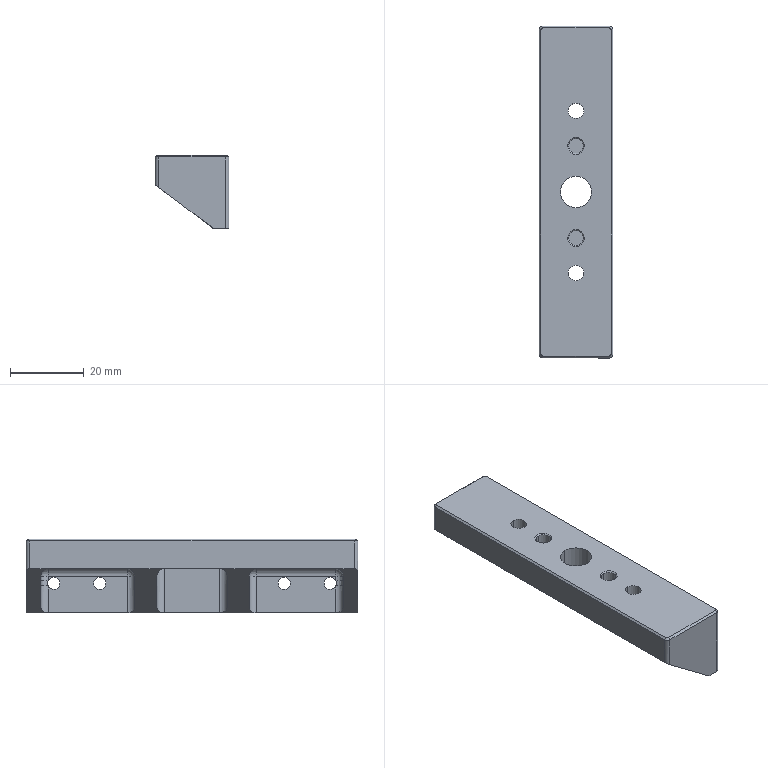NC program | NX | posted with a generic post | part box 20 x 90 x 20 mm
Lines 775 to 1873 of 15930:
(FIXED_CONTOUR , TOOL : D4R0.5)
N1542 T24 M6
N1544 G54
N1546 G17 G0 G90 X-15.314 Y3.135 B0. C0. S9500 M3
N1548 G43 Z30. H24
N1550 Z2.8
N1552 G94 G1 Z1.511 F3000.
N1554 X-15.35 Y3.15 Z1.12
N1556 X-15.455 Y3.194 Z0.745
N1558 X-15.626 Y3.264 Z0.399
N1560 X-15.856 Y3.359 Z0.096
N1562 X-16.136 Y3.474 Z-0.152
N1564 X-16.455 Y3.606 Z-0.337
N1566 X-16.802 Y3.749 Z-0.451
N1568 X-17.163 Y3.898 Z-0.489
N1570 X-17.219 Y3.921
N1572 X-17.486 Y3.991
N1574 X-17.57 Y3.999
N1576 X-17.571 Y4.
N1578 X-38.921 Y4.001
N1580 X-39.024 Y3.998
N1582 X-39.332 Y3.895
N1584 X-39.377 Y3.827 Z-0.589
N1586 X-39.009 Y3.997
N1588 X-38.921 Y4.
N1590 X-17.589
N1592 X-17.5 Y3.998
N1594 X-17.449 Y3.979
N1596 X-17.116 Y3.827
N1598 X-17.095 Y3.764 Z-0.688
N1600 X-17.5 Y3.998
N1602 X-17.589 Y4.
N1604 X-38.97
N1606 X-39.018 Y3.988
N1608 X-39.412 Y3.76
N1610 X-39.426 Y3.696 Z-0.788
N1612 X-39.397 Y3.715
N1614 X-39.014 Y3.987
N1616 X-38.998 Y3.996
N1618 X-38.921 Y4.
N1620 X-17.589
N1622 X-17.5 Y3.998
N1624 X-17.112 Y3.721
N1626 X-17.077 Y3.698
N1628 X-17.072 Y3.636 Z-0.887
N1630 X-17.168 Y3.71
N1632 X-17.5 Y3.998
N1634 X-17.589 Y4.
N1636 X-38.921
N1638 X-38.998 Y3.996
N1640 X-39.405 Y3.655
N1642 X-39.436 Y3.633
N1644 X-39.433 Y3.574 Z-0.987
N1646 X-39.012 Y3.981
N1648 X-38.997 Y3.996
N1650 X-38.921 Y4.
N1652 X-17.589
N1654 X-17.5 Y3.998
N1656 X-17.095 Y3.599
N1658 X-17.068 Y3.575
N1660 X-17.07 Y3.513 Z-1.086
N1662 X-17.095 Y3.536
N1664 X-17.303 Y3.753
N1666 X-17.5 Y3.998
N1668 X-17.589 Y4.
N1670 X-38.921
N1672 X-38.997 Y3.996
N1674 X-39.392 Y3.549
N1676 X-39.408 Y3.533
N1678 X-39.384 Y3.492 Z-1.186
N1680 X-39.178 Y3.737
N1682 X-38.997 Y3.996
N1684 X-38.921 Y4.
N1686 X-17.589
N1688 X-17.5 Y3.998
N1690 X-17.318 Y3.735
N1692 X-17.107 Y3.483
N1694 X-17.127 Y3.467 Z-1.236
N1696 X-17.144 Y3.453 Z-1.285
N1698 X-17.339 Y3.72
N1700 X-17.5 Y3.998
N1702 X-17.589 Y4.
N1704 X-38.921
N1706 X-38.997 Y3.996
N1708 X-39.167 Y3.714
N1710 X-39.359 Y3.449
N1712 X-39.331 Y3.408 Z-1.385
N1714 X-39.15 Y3.697
N1716 X-38.996 Y3.996
N1718 X-38.921 Y4.
N1720 X-17.589
N1722 X-17.5 Y3.998
N1724 X-17.356 Y3.708
N1726 X-17.178 Y3.426
N1728 X-17.198 Y3.41 Z-1.434
N1730 X-17.213 Y3.398 Z-1.484
N1732 X-17.374 Y3.694
N1734 X-17.5 Y3.998
N1736 X-17.589 Y4.
N1738 X-38.921
N1740 X-38.997 Y3.996
N1742 X-39.129 Y3.683
N1744 X-39.294 Y3.384
N1746 X-39.274 Y3.371 Z-1.534
N1748 X-39.256 Y3.359 Z-1.584
N1750 X-39.109 Y3.672
N1752 X-38.997 Y3.996
N1754 X-38.921 Y4.
N1756 X-17.589
N1758 X-17.5 Y3.998
N1760 X-17.393 Y3.681
N1762 X-17.25 Y3.368
N1764 X-17.269 Y3.352 Z-1.633
N1766 X-17.286 Y3.339 Z-1.683
N1768 X-17.297 Y3.361
N1770 X-17.414 Y3.667
N1772 X-17.5 Y3.998
N1774 X-17.589 Y4.
N1776 X-38.921
N1778 X-38.997 Y3.996
N1780 X-39.086 Y3.659
N1782 X-39.206 Y3.354
N1784 X-39.215 Y3.333
N1786 X-39.194 Y3.32 Z-1.733
N1788 X-39.176 Y3.308 Z-1.783
N1790 X-39.167 Y3.329
N1792 X-39.064 Y3.647
N1794 X-38.997 Y3.995
N1796 X-38.921 Y4.
N1798 X-17.589
N1800 X-17.5 Y3.998
N1802 X-17.436 Y3.652
N1804 X-17.333 Y3.332
N1806 X-17.324 Y3.309
N1808 X-17.322 Y3.181 Z-1.882
N1810 X-17.352 Y3.261
N1812 X-17.451 Y3.616
N1814 X-17.5 Y3.998
N1816 X-17.589 Y4.
N1818 X-38.921
N1820 X-38.997 Y3.995
N1822 X-38.998 Y3.976
N1824 X-39.049 Y3.613
N1826 X-39.148 Y3.26
N1828 X-39.177 Y3.183
N1830 Y3.05 Z-1.982
N1832 X-39.148 Y3.128
N1834 X-39.038 Y3.546
N1836 X-38.997 Y3.976
N1838 Y3.995
N1840 X-38.921 Y4.
N1842 X-17.589
N1844 X-17.5 Y3.998
N1846 Y3.982
N1848 X-17.461 Y3.549
N1850 X-17.352 Y3.128
N1852 X-17.322 Y3.048
N1854 X-17.321 Y2.916 Z-2.081
N1856 X-17.352 Y3.
N1858 X-17.442 Y3.32
N1860 X-17.492 Y3.649
N1862 X-17.5 Y3.998
N1864 X-17.589 Y4.
N1866 X-38.921
N1868 X-38.997 Y3.995
N1870 X-39.016 Y3.613
N1872 X-39.074 Y3.255
N1874 X-39.148 Y2.99
N1876 X-39.175 Y2.916
N1878 X-39.174 Y2.783 Z-2.181
N1880 X-39.148 Y2.854
N1882 X-39.046 Y3.255
N1884 X-39.008 Y3.615
N1886 X-38.997 Y3.995
N1888 X-38.921 Y4.
N1890 X-17.589
N1892 X-17.5 Y3.998
N1894 X-17.497 Y3.607
N1896 X-17.447 Y3.235
N1898 X-17.352 Y2.872
N1900 X-17.321 Y2.784
N1902 X-17.322 Y2.651 Z-2.28
N1904 X-17.352 Y2.732
N1906 X-17.456 Y3.128
N1908 X-17.498 Y3.535
N1910 X-17.5 Y3.998
N1912 X-17.589 Y4.
N1914 X-38.921
N1916 X-38.997 Y3.995
N1918 X-39.005 Y3.535
N1920 X-39.045 Y3.127
N1922 X-39.148 Y2.731
N1924 X-39.177 Y2.652
N1926 X-39.175 Y2.519 Z-2.38
N1928 X-39.148 Y2.591
N1930 X-39.059 Y2.918
N1932 X-39.016 Y3.255
N1934 X-38.997 Y3.995
N1936 X-38.921 Y4.
N1938 X-17.589
N1940 X-17.5 Y3.998
N1942 X-17.487 Y3.255
N1944 X-17.441 Y2.92
N1946 X-17.352 Y2.594
N1948 X-17.323 Y2.516
N1950 X-17.322 Y2.385 Z-2.479
N1952 X-17.352 Y2.466
N1954 X-17.455 Y2.855
N1956 X-17.498 Y3.255
N1958 X-17.5 Y3.998
N1960 X-17.589 Y4.
N1962 X-38.921
N1964 X-38.996 Y3.995
N1966 X-39.006 Y3.255
N1968 X-39.046 Y2.854
N1970 X-39.148 Y2.465
N1972 X-39.177 Y2.386
N1974 X-39.179 Y2.253 Z-2.578
N1976 X-39.148 Y2.341
N1978 X-39.037 Y2.792
N1980 X-38.998 Y3.255
N1982 X-38.996 Y3.995
N1984 X-38.921 Y4.
N1986 X-17.589
N1988 X-17.5 Y3.998
N1990 X-17.498 Y3.255
N1992 X-17.486 Y2.942
N1994 X-17.437 Y2.633
N1996 X-17.352 Y2.332
N1998 X-17.322 Y2.252
N2000 X-17.321 Y2.121 Z-2.678
N2002 X-17.352 Y2.203
N2004 X-17.46 Y2.625
N2006 X-17.498 Y3.059
N2008 X-17.5 Y3.998
N2010 X-17.589 Y4.
N2012 X-38.921
N2014 X-38.996 Y3.995
N2016 X-39.007 Y2.975
N2018 X-39.047 Y2.581
N2020 X-39.148 Y2.199
N2022 X-39.177 Y2.121
N2024 X-39.179 Y1.988 Z-2.777
N2026 X-39.148 Y2.077
N2028 X-39.038 Y2.52
N2030 X-38.998 Y2.975
N2032 X-38.996 Y3.995
N2034 X-38.921 Y4.
N2036 X-17.589
N2038 X-17.5 Y3.998
N2040 X-17.498 Y2.975
N2042 X-17.485 Y2.667
N2044 X-17.436 Y2.363
N2046 X-17.352 Y2.067
N2048 X-17.322 Y1.987
N2050 X-17.321 Y1.855 Z-2.877
N2052 X-17.352 Y1.938
N2054 X-17.46 Y2.36
N2056 X-17.497 Y2.793
N2058 X-17.5 Y3.998
N2060 X-17.589 Y4.
N2062 X-38.921
N2064 X-38.996 Y3.995
N2066 X-38.997 Y3.335
N2068 X-39.008 Y2.694
N2070 X-39.049 Y2.308
N2072 X-39.148 Y1.933
N2074 X-39.177 Y1.855
N2076 X-39.18 Y1.724 Z-2.976
N2078 X-39.148 Y1.812
N2080 X-39.038 Y2.247
N2082 X-38.998 Y2.694
N2084 X-38.996 Y3.995
N2086 X-38.921 Y4.
N2088 X-17.589
N2090 X-17.5 Y3.998
N2092 X-17.498 Y2.694
N2094 X-17.464 Y2.242
N2096 X-17.352 Y1.802
N2098 X-17.322 Y1.722
N2100 X-17.323 Y1.589 Z-3.076
N2102 X-17.352 Y1.668
N2104 X-17.459 Y2.084
N2106 X-17.496 Y2.512
N2108 X-17.5 Y3.998
N2110 X-17.589 Y4.
N2112 X-38.921
N2114 X-38.996 Y3.995
N2116 X-38.998 Y2.694
N2118 X-39.009 Y2.349
N2120 X-39.06 Y2.007
N2122 X-39.148 Y1.672
N2124 X-39.177 Y1.589
N2126 X-39.175 Y1.457 Z-3.175
N2128 X-39.148 Y1.536
N2130 X-39.04 Y1.969
N2132 X-38.998 Y2.414
N2134 X-38.996 Y3.995
N2136 X-38.921 Y4.
N2138 X-17.589
N2140 X-17.501 Y3.998
N2142 X-17.498 Y2.414
N2144 X-17.463 Y1.97
N2146 X-17.352 Y1.538
N2148 X-17.322 Y1.457
N2150 X-17.323 Y1.323 Z-3.275
N2152 X-17.352 Y1.401
N2154 X-17.461 Y1.827
N2156 X-17.498 Y2.264
N2158 X-17.501 Y3.998
N2160 X-17.589 Y4.
N2162 X-38.921
N2164 X-38.996 Y3.995
N2166 X-38.998 Y2.414
N2168 X-39.01 Y2.074
N2170 X-39.061 Y1.737
N2172 X-39.148 Y1.407
N2174 X-39.177 Y1.324
N2176 X-39.174 Y1.192 Z-3.374
N2178 X-39.148 Y1.262
N2180 X-39.066 Y1.554
N2182 X-39.022 Y1.854
N2184 X-38.998 Y2.212
N2186 X-38.996 Y3.995
N2188 X-38.921 Y4.
N2190 X-17.589
N2192 X-17.501 Y3.998
N2194 X-17.499 Y3.675
N2196 X-17.498 Y2.134
N2198 X-17.461 Y1.698
N2200 X-17.352 Y1.273
N2202 X-17.322 Y1.192
N2204 Y1.059 Z-3.474
N2206 X-17.352 Y1.14
N2208 X-17.461 Y1.566
N2210 X-17.498 Y2.005
N2212 X-17.499 Y3.675
N2214 X-17.501 Y3.998
N2216 X-17.589 Y4.
N2218 X-38.921
N2220 X-38.996 Y3.995
N2222 X-38.998 Y2.134
N2224 X-39.011 Y1.798
N2226 X-39.062 Y1.466
N2228 X-39.148 Y1.141
N2230 X-39.176 Y1.06
N2232 X-39.179 Y0.927 Z-3.573
N2234 X-39.148 Y1.01
N2236 X-39.04 Y1.426
N2238 X-39.001 Y1.854
N2240 X-38.996 Y3.995
N2242 X-38.984 Y3.997
N2244 X-38.921 Y4.
N2246 X-17.589
N2248 X-17.501 Y3.998
N2250 X-17.499 Y3.675
N2252 X-17.498 Y1.854
N2254 X-17.46 Y1.425
N2256 X-17.352 Y1.008
N2258 X-17.322 Y0.927
N2260 X-17.321 Y0.793 Z-3.673
N2262 X-17.352 Y0.878
N2264 X-17.461 Y1.306
N2266 X-17.498 Y1.746
N2268 X-17.499 Y3.675
N2270 X-17.501 Y3.998
N2272 X-17.589 Y4.
N2274 X-38.921
N2276 X-38.984 Y3.997
N2278 X-38.996 Y3.995
N2280 X-38.998 Y1.854
N2282 X-39.012 Y1.523
N2284 X-39.063 Y1.196
N2286 X-39.148 Y0.876
N2288 X-39.176 Y0.794
N2290 X-39.178 Y0.662 Z-3.772
N2292 X-39.148 Y0.742
N2294 X-39.041 Y1.152
N2296 X-39.002 Y1.574
N2298 X-38.996 Y3.995
N2300 X-38.984 Y3.997
N2302 X-38.921 Y4.
N2304 X-17.589
N2306 X-17.501 Y3.998
N2308 X-17.499 Y3.675
N2310 X-17.498 Y1.574
N2312 X-17.459 Y1.153
N2314 X-17.352 Y0.743
N2316 X-17.322 Y0.661
N2318 Y0.528 Z-3.872
N2320 X-17.352 Y0.608
N2322 X-17.461 Y1.037
N2324 X-17.498 Y1.479
N2326 X-17.499 Y3.675
N2328 X-17.501 Y3.998
N2330 X-17.589 Y4.
N2332 X-38.921
N2334 X-38.984 Y3.997
N2336 X-38.996 Y3.995
N2338 X-38.998 Y1.574
N2340 X-39.034 Y1.086
N2342 X-39.148 Y0.61
N2344 X-39.176 Y0.529
N2346 X-39.178 Y0.397 Z-3.971
N2348 X-39.148 Y0.477
N2350 X-39.043 Y0.879
N2352 X-39.003 Y1.294
N2354 X-39. Y2.635
N2356 X-38.996 Y3.995
N2358 X-38.984 Y3.997
N2360 X-38.921 Y4.
N2362 X-17.589
N2364 X-17.501 Y3.998
N2366 X-17.499 Y3.675
N2368 X-17.498 Y1.294
N2370 X-17.458 Y0.88
N2372 X-17.352 Y0.478
N2374 X-17.322 Y0.396
N2376 Y0.264 Z-4.071
N2378 X-17.352 Y0.346
N2380 X-17.461 Y0.773
N2382 X-17.498 Y1.212
N2384 X-17.499 Y3.675
N2386 X-17.501 Y3.998
N2388 X-17.589 Y4.
N2390 X-38.921
N2392 X-38.984 Y3.997
N2394 X-38.996 Y3.995
N2396 X-38.998 Y1.294
N2398 X-39.035 Y0.813
N2400 X-39.148 Y0.344
N2402 X-39.176 Y0.264
N2404 X-39.177 Y0.131 Z-4.17
N2406 X-39.148 Y0.211
N2408 X-39.044 Y0.606
N2410 X-39.005 Y1.014
N2412 X-38.998 Y1.294
N2414 X-38.996 Y3.995
N2416 X-38.984 Y3.997
N2418 X-38.921 Y4.
N2420 X-17.589
N2422 X-17.501 Y3.998
N2424 X-17.499 Y3.675
N2426 X-17.498 Y1.014
N2428 X-17.456 Y0.607
N2430 X-17.352 Y0.212
N2432 X-17.322 Y0.131
N2434 Y-0.003 Z-4.27
N2436 X-17.352 Y0.078
N2438 X-17.438 Y0.383
N2440 X-17.487 Y0.697
N2442 X-17.498 Y1.014
N2444 X-17.499 Y3.675
N2446 X-17.501 Y3.998
N2448 X-17.589 Y4.
N2450 X-38.921
N2452 X-38.984 Y3.997
N2454 X-38.996 Y3.995
N2456 X-38.998 Y1.014
N2458 X-39.036 Y0.543
N2460 X-39.148 Y0.085
N2462 X-39.178 Y-0.001
N2464 X-39.177 Y-0.134 Z-4.369
N2466 X-39.148 Y-0.055
N2468 X-39.046 Y0.334
N2470 X-39.006 Y0.734
N2472 X-38.998 Y1.014
N2474 Y3.99
N2476 X-38.991 Y3.997
N2478 X-38.921 Y4.
N2480 X-17.589
N2482 X-17.501 Y3.998
N2484 X-17.499 Y3.675
N2486 X-17.498 Y0.802
N2488 X-17.461 Y0.367
N2490 X-17.352 Y-0.056
N2492 X-17.322 Y-0.135
N2494 Y-0.268 Z-4.469
N2496 X-17.352 Y-0.188
N2498 X-17.437 Y0.113
N2500 X-17.486 Y0.421
N2502 X-17.498 Y0.734
N2504 X-17.499 Y3.675
N2506 X-17.501 Y3.998
N2508 X-17.589 Y4.
N2510 X-38.921
N2512 X-38.984 Y3.997
N2514 X-38.996 Y3.995
N2516 X-38.998 Y0.734
N2518 X-39.037 Y0.271
N2520 X-39.148 Y-0.179
N2522 X-39.179 Y-0.267
N2524 X-39.176 Y-0.4 Z-4.568
N2526 X-39.148 Y-0.319
N2528 X-39.036 Y0.145
N2530 X-38.998 Y0.62
N2532 X-38.996 Y3.995
N2534 X-38.984 Y3.997
N2536 X-38.921 Y4.
N2538 X-17.589
N2540 X-17.501 Y3.998
N2542 X-17.499 Y3.675
N2544 X-17.497 Y0.546
N2546 X-17.461 Y0.109
N2548 X-17.352 Y-0.316
N2550 X-17.321 Y-0.399
N2552 X-17.322 Y-0.533 Z-4.668
N2554 X-17.352 Y-0.453
N2556 X-17.436 Y-0.157
N2558 X-17.485 Y0.146
N2560 X-17.498 Y0.454
N2562 X-17.499 Y3.675
N2564 X-17.501 Y3.998
N2566 X-17.589 Y4.
N2568 X-38.921
N2570 X-38.984 Y3.997
N2572 X-38.996 Y3.995
N2574 X-38.998 Y0.454
N2576 X-39.038 Y-0.001
N2578 X-39.148 Y-0.443
N2580 X-39.18 Y-0.532
N2582 X-39.177 Y-0.666 Z-4.767
N2584 X-39.148 Y-0.583
N2586 X-39.036 Y-0.118
N2588 X-38.998 Y0.359
N2590 X-38.996 Y3.994
N2592 X-38.984 Y3.997
N2594 X-38.921 Y4.
N2596 X-17.589
N2598 X-17.501 Y3.998
N2600 X-17.499 Y3.675
N2602 X-17.498 Y0.454
N2604 X-17.497 Y0.173
N2606 X-17.452 Y-0.211
N2608 X-17.352 Y-0.586
N2610 X-17.322 Y-0.666
N2612 Y-0.798 Z-4.866
N2614 X-17.352 Y-0.718
N2616 X-17.464 Y-0.279
N2618 X-17.498 Y0.173
N2620 X-17.499 Y3.675
N2622 X-17.501 Y3.998
N2624 X-17.589 Y4.
N2626 X-38.921
N2628 X-38.984 Y3.997
N2630 X-38.996 Y3.994
N2632 X-38.998 Y0.173
N2634 X-39.039 Y-0.278
N2636 X-39.148 Y-0.719
N2638 X-39.176 Y-0.798
N2640 Y-0.93 Z-4.966
N2642 X-39.148 Y-0.848
N2644 X-39.06 Y-0.514
N2646 X-39.01 Y-0.172
N2648 X-38.998 Y0.173
N2650 X-38.996 Y3.994
N2652 X-38.984 Y3.997
N2654 X-38.921 Y4.
N2656 X-17.589
N2658 X-17.501 Y3.998
N2660 X-17.5 Y2.992
N2662 X-17.498 Y0.023
N2664 X-17.461 Y-0.417
N2666 X-17.352 Y-0.845
N2668 X-17.32 Y-0.931
N2670 X-17.322 Y-1.063 Z-5.065
N2672 X-17.352 Y-0.982
N2674 X-17.463 Y-0.551
N2676 X-17.498 Y-0.107
N2678 X-17.5 Y2.96
N2680 X-17.501 Y3.998
N2682 X-17.589 Y4.
N2684 X-38.921
N2686 X-38.984 Y3.997
N2688 X-38.996 Y3.994
N2690 X-38.998 Y-0.107
N2692 X-39.04 Y-0.551
N2694 X-39.148 Y-0.984
N2696 X-39.175 Y-1.063
N2698 X-39.176 Y-1.196 Z-5.165
N2700 X-39.148 Y-1.113
N2702 X-39.061 Y-0.784
N2704 X-39.011 Y-0.447
N2706 X-38.998 Y-0.107
N2708 X-38.996 Y3.994
N2710 X-38.984 Y3.997
N2712 X-38.921 Y4.
N2714 X-17.589
N2716 X-17.501 Y3.998
N2718 X-17.5 Y2.923
N2720 X-17.498 Y-0.253
N2722 X-17.461 Y-0.692
N2724 X-17.352 Y-1.119
N2726 X-17.323 Y-1.197
N2728 X-17.322 Y-1.328 Z-5.264
N2730 X-17.352 Y-1.247
N2732 X-17.461 Y-0.823
N2734 X-17.498 Y-0.387
N2736 X-17.5 Y2.89
N2738 X-17.501 Y3.998
N2740 X-17.589 Y4.
N2742 X-38.921
N2744 X-38.984 Y3.997
N2746 X-38.996 Y3.994
N2748 X-38.999 Y-0.387
N2750 X-39.041 Y-0.824
N2752 X-39.148 Y-1.25
N2754 X-39.175 Y-1.328
N2756 X-39.176 Y-1.46 Z-5.364
N2758 X-39.148 Y-1.379
N2760 X-39.062 Y-1.054
N2762 X-39.012 Y-0.722
N2764 X-38.998 Y-0.387
N2766 X-38.996 Y3.994
N2768 X-38.984 Y3.997
N2770 X-38.921 Y4.
N2772 X-17.589
N2774 X-17.501 Y3.998
N2776 X-17.5 Y2.857
N2778 X-17.498 Y-0.517
N2780 X-17.461 Y-0.954
N2782 X-17.352 Y-1.38
N2784 X-17.322 Y-1.461
N2786 Y-1.593 Z-5.463
N2788 X-17.352 Y-1.512
N2790 X-17.46 Y-1.095
N2792 X-17.498 Y-0.667
N2794 X-17.5 Y2.82
N2796 X-17.501 Y3.998
N2798 X-17.589 Y4.
N2800 X-38.921
N2802 X-38.984 Y3.997
N2804 X-38.996 Y3.994
N2806 X-39. Y0.494
N2808 X-39.001 Y-0.667
N2810 X-39.04 Y-1.095
N2812 X-39.148 Y-1.511
N2814 X-39.179 Y-1.593
N2816 X-39.176 Y-1.726 Z-5.563
N2818 X-39.148 Y-1.645
N2820 X-39.063 Y-1.325
N2822 X-39.012 Y-0.998
N2824 X-38.998 Y-0.667
N2826 X-38.995 Y3.994
N2828 X-38.984 Y3.997
N2830 X-38.921 Y4.
N2832 X-17.589
N2834 X-17.501 Y3.998
N2836 X-17.5 Y2.793
N2838 X-17.498 Y-0.776
N2840 X-17.461 Y-1.215
N2842 X-17.352 Y-1.642
N2844 X-17.321 Y-1.727
N2846 X-17.322 Y-1.859 Z-5.662
N2848 X-17.352 Y-1.777
N2850 X-17.459 Y-1.368
N2852 X-17.498 Y-0.947
N2854 X-17.5 Y2.134
N2856 X-17.501 Y2.75
N2858 Y3.998
N2860 X-17.589 Y4.
N2862 X-38.921
N2864 X-38.984 Y3.997
N2866 X-38.995 Y3.994
N2868 X-39. Y0.899
N2870 X-39.002 Y-0.947
N2872 X-39.041 Y-1.368
N2874 X-39.148 Y-1.778
N2876 X-39.178 Y-1.858
N2878 X-39.176 Y-1.991 Z-5.762
N2880 X-39.148 Y-1.91
N2882 X-39.034 Y-1.435
N2884 X-38.998 Y-0.947
N2886 X-38.995 Y3.994
N2888 X-38.984 Y3.997
N2890 X-38.921 Y4.
N2892 X-17.589
N2894 X-17.501 Y3.998
N2896 Y2.726
N2898 X-17.5 Y2.098
N2900 X-17.498 Y-1.043
N2902 X-17.461 Y-1.484
N2904 X-17.352 Y-1.912
N2906 X-17.323 Y-1.993
N2908 X-17.322 Y-2.124 Z-5.861
N2910 X-17.352 Y-2.042
N2912 X-17.458 Y-1.641
N2914 X-17.498 Y-1.227
N2916 X-17.5 Y2.029
N2918 X-17.501 Y2.68
N2920 Y3.998
N2922 X-17.589 Y4.
N2924 X-38.921
N2926 X-38.984 Y3.997
N2928 X-38.995 Y3.994
N2930 X-38.998 Y-0.947
N2932 X-39.004 Y-1.227
N2934 X-39.043 Y-1.641
N2936 X-39.148 Y-2.044
N2938 X-39.178 Y-2.123
N2940 X-39.176 Y-2.257 Z-5.961
N2942 X-39.148 Y-2.176
N2944 X-39.035 Y-1.708
N2946 X-38.998 Y-1.227
N2948 X-38.995 Y3.994
N2950 X-38.984 Y3.997
N2952 X-38.921 Y4.
N2954 X-17.589
N2956 X-17.501 Y3.998
N2958 Y2.659
N2960 X-17.5 Y1.998
N2962 X-17.498 Y-1.309
N2964 X-17.461 Y-1.748
N2966 X-17.352 Y-2.174
N2968 X-17.322 Y-2.256
N2970 Y-2.389 Z-6.06
N2972 X-17.352 Y-2.308
N2974 X-17.456 Y-1.913
N2976 X-17.498 Y-1.507
N2978 X-17.5 Y1.924
N2980 X-17.501 Y2.61
N2982 Y3.998
N2984 X-17.589 Y4.
N2986 X-38.921
N2988 X-38.99 Y3.996
N2990 X-38.997 Y3.989
N2992 X-38.998 Y-1.227
N2994 X-39.005 Y-1.507
N2996 X-39.044 Y-1.914
N2998 X-39.148 Y-2.31
N3000 X-39.177 Y-2.389
N3002 X-39.178 Y-2.521 Z-6.16
N3004 X-39.148 Y-2.435
N3006 X-39.036 Y-1.977
N3008 X-38.998 Y-1.507
N3010 X-38.995 Y3.994
N3012 X-38.984 Y3.997
N3014 X-38.921 Y4.
N3016 X-17.589
N3018 X-17.501 Y3.998
N3020 X-17.5 Y1.924
N3022 X-17.498 Y-1.507
N3024 X-17.487 Y-1.824
N3026 X-17.438 Y-2.137
N3028 X-17.352 Y-2.442
N3030 X-17.322 Y-2.523
N3032 X-17.323 Y-2.655 Z-6.259
N3034 X-17.352 Y-2.576
N3036 X-17.461 Y-2.154
N3038 X-17.498 Y-1.719
N3040 X-17.5 Y1.844
N3042 X-17.501 Y2.557
N3044 Y3.998
N3046 X-17.589 Y4.
N3048 X-38.921
N3050 X-38.984 Y3.997
N3052 X-38.995 Y3.994
N3054 X-38.998 Y-1.638
N3056 X-39.036 Y-2.112
N3058 X-39.148 Y-2.574
N3060 X-39.176 Y-2.655
N3062 X-39.179 Y-2.787 Z-6.359
N3064 X-39.148 Y-2.699
N3066 X-39.037 Y-2.249
N3068 X-38.998 Y-1.787
N3070 X-38.995 Y3.994
N3072 X-38.984 Y3.997
N3074 X-38.921 Y4.
N3076 X-17.589
N3078 X-17.501 Y3.998
N3080 X-17.5 Y1.819
N3082 X-17.498 Y-1.787
N3084 X-17.486 Y-2.099
N3086 X-17.437 Y-2.408
N3088 X-17.352 Y-2.708
N3090 X-17.322 Y-2.788
N3092 Y-2.92 Z-6.458
N3094 X-17.352 Y-2.84
N3096 X-17.454 Y-2.459
N3098 X-17.497 Y-2.068
N3100 X-17.5 Y1.819
N3102 X-17.501 Y3.998
N3104 X-17.589 Y4.
N3106 X-38.921
N3108 X-38.984 Y3.997
N3110 X-38.995 Y3.994
N3112 X-38.998 Y-1.899
N3114 X-39.036 Y-2.375
N3116 X-39.148 Y-2.839
N3118 X-39.176 Y-2.92
N3120 X-39.18 Y-3.052 Z-6.558
N3122 X-39.148 Y-2.963
N3124 X-39.038 Y-2.521
N3126 X-38.998 Y-2.068
N3128 X-38.995 Y3.994
N3130 X-38.984 Y3.997
N3132 X-38.921 Y4.
N3134 X-17.589
N3136 X-17.502 Y3.998
N3138 X-17.5 Y1.714
N3140 X-17.498 Y-2.068
N3142 X-17.485 Y-2.374
N3144 X-17.436 Y-2.678
N3146 X-17.352 Y-2.973
N3148 X-17.322 Y-3.053
N3150 Y-3.186 Z-6.657
N3152 X-17.352 Y-3.106
N3154 X-17.452 Y-2.732
N3156 X-17.497 Y-2.348
N3158 X-17.499 Y-1.311
N3160 X-17.5 Y1.714
N3162 X-17.502 Y3.998
N3164 X-17.589 Y4.
N3166 X-38.921
N3168 X-38.984 Y3.997
N3170 X-38.995 Y3.994
N3172 X-38.998 Y-2.161
N3174 X-39.036 Y-2.638
N3176 X-39.148 Y-3.103
N3178 X-39.176 Y-3.185
N3180 Y-3.318 Z-6.757
N3182 X-39.148 Y-3.239
N3184 X-39.039 Y-2.799
N3186 X-38.998 Y-2.348
N3188 X-38.995 Y3.994
N3190 X-38.984 Y3.997
N3192 X-38.921 Y4.
N3194 X-17.589
N3196 X-17.502 Y3.998
N3198 X-17.501 Y1.592
N3200 X-17.5 Y0.804
N3202 X-17.498 Y-2.348
N3204 X-17.464 Y-2.799
N3206 X-17.352 Y-3.238
N3208 X-17.322 Y-3.318
N3210 X-17.321 Y-3.451 Z-6.856
N3212 X-17.352 Y-3.365
N3214 X-17.461 Y-2.937
N3216 X-17.498 Y-2.497
N3218 X-17.5 Y0.729
N3220 X-17.501 Y1.535
N3222 X-17.502 Y3.998
N3224 X-17.589 Y4.
N3226 X-38.921
N3228 X-38.984 Y3.997
N3230 X-38.995 Y3.994
N3232 X-38.998 Y-2.348
N3234 X-39.01 Y-2.693
N3236 X-39.06 Y-3.034
N3238 X-39.148 Y-3.368
N3240 X-39.176 Y-3.451
N3242 Y-3.583 Z-6.956
N3244 X-39.148 Y-3.505
N3246 X-39.04 Y-3.072
N3248 X-38.998 Y-2.628
N3250 X-38.995 Y3.994
N3252 X-38.984 Y3.997
N3254 X-38.921 Y4.
N3256 X-17.589
N3258 X-17.502 Y3.998
N3260 X-17.5 Y0.664
N3262 X-17.498 Y-2.628
N3264 X-17.462 Y-3.071
N3266 X-17.352 Y-3.502
N3268 X-17.322 Y-3.583
N3270 X-17.323 Y-3.717 Z-7.055
N3272 X-17.352 Y-3.639
N3274 X-17.461 Y-3.212
N3276 X-17.498 Y-2.773
N3278 X-17.5 Y0.591
N3280 X-17.502 Y3.998
N3282 X-17.589 Y4.
N3284 X-38.921
N3286 X-38.984 Y3.997
N3288 X-38.995 Y3.994
N3290 X-38.998 Y-2.628
N3292 X-39.011 Y-2.968
N3294 X-39.061 Y-3.304
N3296 X-39.148 Y-3.633
N3298 X-39.177 Y-3.716
N3300 X-39.175 Y-3.849 Z-7.154
N3302 X-39.148 Y-3.771
N3304 X-39.041 Y-3.345
N3306 X-39. Y-2.908
N3308 X-38.998 Y-1.802
N3310 X-38.995 Y3.994
N3312 X-38.984 Y3.997
N3314 X-38.921 Y4.
N3316 X-17.589
N3318 X-17.502 Y3.998
N3320 X-17.5 Y0.524
N3322 X-17.498 Y-2.908
N3324 X-17.461 Y-3.343
N3326 X-17.352 Y-3.767
N3328 X-17.322 Y-3.848
N3330 Y-3.981 Z-7.254
N3332 X-17.352 Y-3.898
N3334 X-17.454 Y-3.504
N3336 X-17.494 Y-3.099
N3338 X-17.498 Y-2.908
N3340 X-17.5 Y0.524
N3342 X-17.502 Y3.998
N3344 X-17.589 Y4.
N3346 X-38.921
N3348 X-38.984 Y3.997
N3350 X-38.995 Y3.994
N3352 X-38.998 Y-2.908
N3354 X-39.012 Y-3.243
N3356 X-39.062 Y-3.575
N3358 X-39.148 Y-3.899
N3360 X-39.177 Y-3.982
N3362 X-39.179 Y-4.114 Z-7.353
N3364 X-39.148 Y-4.031
N3366 X-39.04 Y-3.616
N3368 X-39.001 Y-3.188
N3370 X-38.999 Y-0.503
N3372 X-38.996 Y3.976
N3374 X-38.995 Y3.994
N3376 X-38.984 Y3.997
N3378 X-38.921 Y4.
N3380 X-17.589
N3382 X-17.502 Y3.998
N3384 X-17.5 Y0.384
N3386 X-17.498 Y-3.188
N3388 X-17.46 Y-3.616
N3390 X-17.352 Y-4.032
N3392 X-17.322 Y-4.113
N3394 X-17.321 Y-4.247 Z-7.453
N3396 X-17.352 Y-4.162
N3398 X-17.461 Y-3.735
N3400 X-17.498 Y-3.295
N3402 X-17.5 Y0.33
N3404 X-17.502 Y3.998
N3406 X-17.589 Y4.
N3408 X-38.921
N3410 X-38.984 Y3.997
N3412 X-38.995 Y3.994
N3414 X-38.997 Y3.971
N3416 X-38.998 Y-3.188
N3418 X-39.013 Y-3.518
N3420 X-39.063 Y-3.845
N3422 X-39.148 Y-4.165
N3424 X-39.176 Y-4.246
N3426 X-39.178 Y-4.378 Z-7.552
N3428 X-39.148 Y-4.298
N3430 X-39.041 Y-3.889
N3432 X-39.002 Y-3.468
N3434 X-39. Y-0.676
N3436 X-38.995 Y3.994
N3438 X-38.984 Y3.997
N3440 X-38.921 Y4.
N3442 X-17.589
N3444 X-17.502 Y3.998
N3446 X-17.5 Y0.243
N3448 X-17.498 Y-3.468
N3450 X-17.459 Y-3.888
N3452 X-17.352 Y-4.297
N3454 X-17.322 Y-4.379
N3456 X-17.323 Y-4.513 Z-7.652
N3458 X-17.352 Y-4.432
N3460 X-17.461 Y-4.004
N3462 X-17.498 Y-3.563
N3464 X-17.5 Y0.196
N3466 X-17.502 Y3.998
N3468 X-17.589 Y4.
N3470 X-38.921
N3472 X-38.984 Y3.996
N3474 X-38.995 Y3.994
N3476 X-38.997 Y3.971
N3478 X-38.998 Y-3.468
N3480 X-39.034 Y-3.955
N3482 X-39.148 Y-4.431
N3484 X-39.176 Y-4.512
N3486 X-39.178 Y-4.644 Z-7.751
N3488 X-39.148 Y-4.564
N3490 X-39.043 Y-4.162
N3492 X-39.004 Y-3.748
N3494 X-38.998 Y-3.468
N3496 X-38.997 Y3.983
N3498 X-38.984 Y3.996
N3500 X-38.921 Y4.
N3502 X-17.589
N3504 X-17.502 Y3.998
N3506 X-17.5 Y0.103
N3508 X-17.498 Y-3.748
N3510 X-17.457 Y-4.161
N3512 X-17.352 Y-4.562
N3514 X-17.322 Y-4.644
N3516 Y-4.777 Z-7.851
N3518 X-17.352 Y-4.694
N3520 X-17.461 Y-4.268
N3522 X-17.498 Y-3.829
N3524 X-17.5 Y0.063
N3526 X-17.502 Y3.998
N3528 X-17.589 Y4.
N3530 X-38.921
N3532 X-38.984 Y3.996
N3534 X-38.995 Y3.993
N3536 X-38.997 Y3.971
N3538 X-38.998 Y-3.748
N3540 X-39.035 Y-4.228
N3542 X-39.148 Y-4.696
N3544 X-39.176 Y-4.777
N3546 X-39.177 Y-4.909 Z-7.95
N3548 X-39.148 Y-4.83
N3550 X-39.045 Y-4.435
N3552 X-39.005 Y-4.028
N3554 X-38.998 Y-3.748
N3556 X-38.997 Y3.983
N3558 X-38.984 Y3.996
N3560 X-38.921 Y4.
N3562 X-17.589
N3564 X-17.502 Y3.998
N3566 X-17.5 Y-0.037
N3568 X-17.498 Y-4.028
N3570 X-17.456 Y-4.434
N3572 X-17.352 Y-4.828
N3574 X-17.322 Y-4.909
N3576 Y-5.043 Z-8.05
N3578 X-17.352 Y-4.962
N3580 X-17.438 Y-4.658
N3582 X-17.487 Y-4.345
N3584 X-17.498 Y-4.028
N3586 X-17.5 Y-0.037
N3588 X-17.502 Y3.998
N3590 X-17.589 Y4.
N3592 X-38.921
N3594 X-38.984 Y3.996
N3596 X-38.995 Y3.993
N3598 X-38.996 Y3.971
N3600 X-38.998 Y-4.028
N3602 X-39.036 Y-4.498
N3604 X-39.148 Y-4.955
N3606 X-39.178 Y-5.041
N3608 X-39.176 Y-5.176 Z-8.149
N3610 X-39.148 Y-5.095
N3612 X-39.036 Y-4.632
N3614 X-38.998 Y-4.157
N3616 X-38.996 Y3.976
N3618 X-38.995 Y3.993
N3620 X-38.984 Y3.996
N3622 X-38.921 Y4.
N3624 X-17.589
N3626 X-17.502 Y3.998
N3628 X-17.5 Y-0.142
N3630 X-17.498 Y-4.239
N3632 X-17.461 Y-4.674
N3634 X-17.352 Y-5.096
N3636 X-17.323 Y-5.176
N3638 X-17.322 Y-5.308 Z-8.249
N3640 X-17.352 Y-5.228
N3642 X-17.437 Y-4.928
N3644 X-17.486 Y-4.62
N3646 X-17.498 Y-4.309
N3648 X-17.5 Y3.675
N3650 X-17.502 Y3.998
N3652 X-17.589 Y4.
N3654 X-38.921
N3656 X-38.984 Y3.996
N3658 X-38.995 Y3.993
N3660 X-38.996 Y3.971
N3662 X-38.998 Y-4.309
N3664 X-39.037 Y-4.77
N3666 X-39.148 Y-5.219
N3668 X-39.179 Y-5.308
N3670 X-39.176 Y-5.441 Z-8.348
N3672 X-39.148 Y-5.359
N3674 X-39.036 Y-4.894
N3676 X-38.998 Y-4.418
N3678 X-38.996 Y3.976
N3680 X-38.995 Y3.993
N3682 X-38.984 Y3.996
N3684 X-38.921 Y4.
N3686 X-17.589
N3688 X-17.502 Y3.998
N3690 X-17.5 Y0.803
N3692 X-17.497 Y-4.495
N3694 X-17.461 Y-4.931
N3696 X-17.352 Y-5.356
N3698 X-17.321 Y-5.441
N3700 X-17.322 Y-5.573 Z-8.448
N3702 X-17.352 Y-5.493
N3704 X-17.436 Y-5.198
N3706 X-17.485 Y-4.895
N3708 X-17.498 Y-4.589
N3710 X-17.5 Y-0.303
N3712 X-17.502 Y3.998
N3714 X-17.589 Y4.
N3716 X-38.921
N3718 X-38.984 Y3.996
N3720 X-38.995 Y3.993
N3722 X-38.996 Y3.971
N3724 X-38.998 Y-4.589
N3726 X-39.038 Y-5.042
N3728 X-39.148 Y-5.484
N3730 X-39.18 Y-5.572
N3732 X-39.176 Y-5.706 Z-8.547